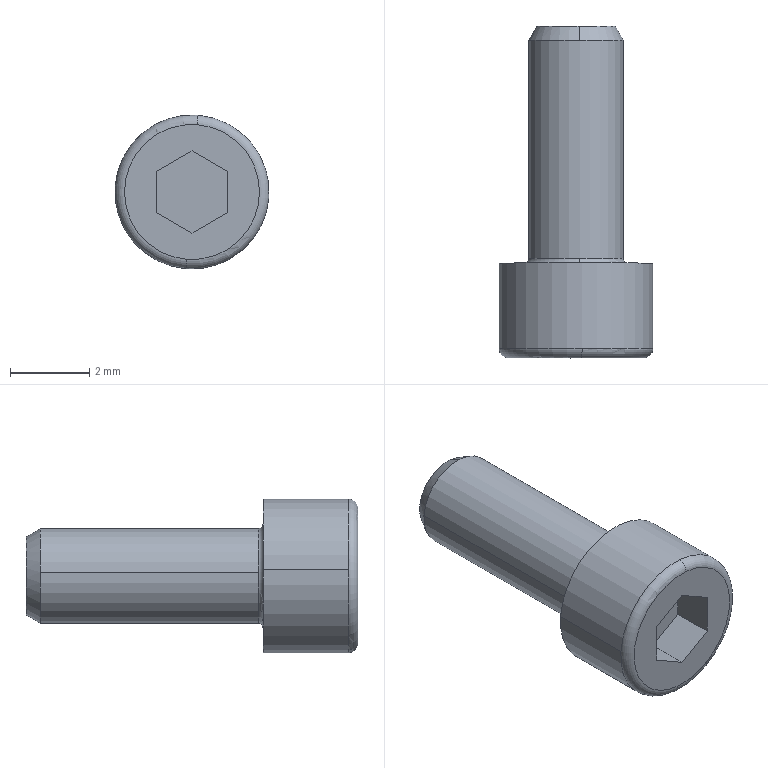Part | STEP file | 2026.6.15-Main Assembly图.sldasm-Part-277 | 1 solid | 20 faces | box 3.9 x 8.4 x 3.9 mm | volume 52.478 mm3 | plane 10 | torus 4 | cylinder 4 | cone 2 | commonest cylinder face diameters 2.4 x2 3.9 x2
STEP:
#1=CARTESIAN_POINT('',(-1526.09,1420.064,3413.556));
#2=VERTEX_POINT('',#1);
#3=CARTESIAN_POINT('',(-1526.09,1420.064,3412.517));
#4=VERTEX_POINT('',#3);
#5=CARTESIAN_POINT('',(-1526.09,1420.064,3413.556));
#6=DIRECTION('',(0.,0.,-1.));
#7=VECTOR('',#6,1000.);
#8=LINE('',#5,#7);
#9=EDGE_CURVE('',#2,#4,#8,.T.);
#10=ORIENTED_EDGE('',*,*,#9,.T.);
#11=CARTESIAN_POINT('',(-1525.19,1420.064,3411.997));
#12=VERTEX_POINT('',#11);
#13=CARTESIAN_POINT('',(-1526.09,1420.064,3412.517));
#14=DIRECTION('',(0.866,0.,-0.5));
#15=VECTOR('',#14,1000.);
#16=LINE('',#13,#15);
#17=EDGE_CURVE('',#4,#12,#16,.T.);
#18=ORIENTED_EDGE('',*,*,#17,.T.);
#19=CARTESIAN_POINT('',(-1524.29,1420.064,3412.517));
#20=VERTEX_POINT('',#19);
#21=CARTESIAN_POINT('',(-1525.19,1420.064,3411.997));
#22=DIRECTION('',(0.866,0.,0.5));
#23=VECTOR('',#22,1000.);
#24=LINE('',#21,#23);
#25=EDGE_CURVE('',#12,#20,#24,.T.);
#26=ORIENTED_EDGE('',*,*,#25,.T.);
#27=CARTESIAN_POINT('',(-1524.29,1420.064,3413.556));
#28=VERTEX_POINT('',#27);
#29=CARTESIAN_POINT('',(-1524.29,1420.064,3412.517));
#30=DIRECTION('',(0.,0.,1.));
#31=VECTOR('',#30,1000.);
#32=LINE('',#29,#31);
#33=EDGE_CURVE('',#20,#28,#32,.T.);
#34=ORIENTED_EDGE('',*,*,#33,.T.);
#35=CARTESIAN_POINT('',(-1525.19,1420.064,3414.076));
#36=VERTEX_POINT('',#35);
#37=CARTESIAN_POINT('',(-1524.29,1420.064,3413.556));
#38=DIRECTION('',(-0.866,0.,0.5));
#39=VECTOR('',#38,1000.);
#40=LINE('',#37,#39);
#41=EDGE_CURVE('',#28,#36,#40,.T.);
#42=ORIENTED_EDGE('',*,*,#41,.T.);
#43=CARTESIAN_POINT('',(-1525.19,1420.064,3414.076));
#44=DIRECTION('',(-0.866,0.,-0.5));
#45=VECTOR('',#44,1000.);
#46=LINE('',#43,#45);
#47=EDGE_CURVE('',#36,#2,#46,.T.);
#48=ORIENTED_EDGE('',*,*,#47,.T.);
#49=EDGE_LOOP('',(#10,#18,#26,#34,#42,#48));
#50=FACE_OUTER_BOUND('',#49,.T.);
#51=CARTESIAN_POINT('',(-1523.39,1420.064,3413.036));
#52=DIRECTION('',(0.,1.,0.));
#53=DIRECTION('',(0.,0.,-1.));
#54=AXIS2_PLACEMENT_3D('',#51,#52,#53);
#55=PLANE('',#54);
#56=ADVANCED_FACE('',(#50),#55,.F.);
#57=ORIENTED_EDGE('',*,*,#9,.F.);
#58=CARTESIAN_POINT('',(-1526.09,1419.014,3413.556));
#59=VERTEX_POINT('',#58);
#60=CARTESIAN_POINT('',(-1526.09,1420.064,3413.556));
#61=DIRECTION('',(0.,-1.,0.));
#62=VECTOR('',#61,1000.);
#63=LINE('',#60,#62);
#64=EDGE_CURVE('',#2,#59,#63,.T.);
#65=ORIENTED_EDGE('',*,*,#64,.T.);
#66=CARTESIAN_POINT('',(-1526.09,1419.014,3412.517));
#67=VERTEX_POINT('',#66);
#68=CARTESIAN_POINT('',(-1526.09,1419.014,3412.517));
#69=DIRECTION('',(0.,0.,1.));
#70=VECTOR('',#69,1000.);
#71=LINE('',#68,#70);
#72=EDGE_CURVE('',#67,#59,#71,.T.);
#73=ORIENTED_EDGE('',*,*,#72,.F.);
#74=CARTESIAN_POINT('',(-1526.09,1420.064,3412.517));
#75=DIRECTION('',(0.,1.,0.));
#76=VECTOR('',#75,1000.);
#77=LINE('',#74,#76);
#78=EDGE_CURVE('',#67,#4,#77,.T.);
#79=ORIENTED_EDGE('',*,*,#78,.T.);
#80=EDGE_LOOP('',(#57,#65,#73,#79));
#81=FACE_OUTER_BOUND('',#80,.T.);
#82=CARTESIAN_POINT('',(-1526.09,1420.064,3413.556));
#83=DIRECTION('',(-1.,0.,0.));
#84=DIRECTION('',(0.,0.,1.));
#85=AXIS2_PLACEMENT_3D('',#82,#83,#84);
#86=PLANE('',#85);
#87=ADVANCED_FACE('',(#81),#86,.F.);
#88=ORIENTED_EDGE('',*,*,#47,.F.);
#89=CARTESIAN_POINT('',(-1525.19,1419.014,3414.076));
#90=VERTEX_POINT('',#89);
#91=CARTESIAN_POINT('',(-1525.19,1420.064,3414.076));
#92=DIRECTION('',(0.,-1.,0.));
#93=VECTOR('',#92,1000.);
#94=LINE('',#91,#93);
#95=EDGE_CURVE('',#36,#90,#94,.T.);
#96=ORIENTED_EDGE('',*,*,#95,.T.);
#97=CARTESIAN_POINT('',(-1526.09,1419.014,3413.556));
#98=DIRECTION('',(0.866,0.,0.5));
#99=VECTOR('',#98,1000.);
#100=LINE('',#97,#99);
#101=EDGE_CURVE('',#59,#90,#100,.T.);
#102=ORIENTED_EDGE('',*,*,#101,.F.);
#103=ORIENTED_EDGE('',*,*,#64,.F.);
#104=EDGE_LOOP('',(#88,#96,#102,#103));
#105=FACE_OUTER_BOUND('',#104,.T.);
#106=CARTESIAN_POINT('',(-1525.19,1420.064,3414.076));
#107=DIRECTION('',(-0.5,0.,0.866));
#108=DIRECTION('',(0.,1.,0.));
#109=AXIS2_PLACEMENT_3D('',#106,#107,#108);
#110=PLANE('',#109);
#111=ADVANCED_FACE('',(#105),#110,.F.);
#112=ORIENTED_EDGE('',*,*,#41,.F.);
#113=CARTESIAN_POINT('',(-1524.29,1419.014,3413.556));
#114=VERTEX_POINT('',#113);
#115=CARTESIAN_POINT('',(-1524.29,1420.064,3413.556));
#116=DIRECTION('',(0.,-1.,0.));
#117=VECTOR('',#116,1000.);
#118=LINE('',#115,#117);
#119=EDGE_CURVE('',#28,#114,#118,.T.);
#120=ORIENTED_EDGE('',*,*,#119,.T.);
#121=CARTESIAN_POINT('',(-1525.19,1419.014,3414.076));
#122=DIRECTION('',(0.866,0.,-0.5));
#123=VECTOR('',#122,1000.);
#124=LINE('',#121,#123);
#125=EDGE_CURVE('',#90,#114,#124,.T.);
#126=ORIENTED_EDGE('',*,*,#125,.F.);
#127=ORIENTED_EDGE('',*,*,#95,.F.);
#128=EDGE_LOOP('',(#112,#120,#126,#127));
#129=FACE_OUTER_BOUND('',#128,.T.);
#130=CARTESIAN_POINT('',(-1524.29,1420.064,3413.556));
#131=DIRECTION('',(0.5,0.,0.866));
#132=DIRECTION('',(-0.866,0.,0.5));
#133=AXIS2_PLACEMENT_3D('',#130,#131,#132);
#134=PLANE('',#133);
#135=ADVANCED_FACE('',(#129),#134,.F.);
#136=ORIENTED_EDGE('',*,*,#33,.F.);
#137=CARTESIAN_POINT('',(-1524.29,1419.014,3412.517));
#138=VERTEX_POINT('',#137);
#139=CARTESIAN_POINT('',(-1524.29,1420.064,3412.517));
#140=DIRECTION('',(0.,-1.,0.));
#141=VECTOR('',#140,1000.);
#142=LINE('',#139,#141);
#143=EDGE_CURVE('',#20,#138,#142,.T.);
#144=ORIENTED_EDGE('',*,*,#143,.T.);
#145=CARTESIAN_POINT('',(-1524.29,1419.014,3413.556));
#146=DIRECTION('',(0.,0.,-1.));
#147=VECTOR('',#146,1000.);
#148=LINE('',#145,#147);
#149=EDGE_CURVE('',#114,#138,#148,.T.);
#150=ORIENTED_EDGE('',*,*,#149,.F.);
#151=ORIENTED_EDGE('',*,*,#119,.F.);
#152=EDGE_LOOP('',(#136,#144,#150,#151));
#153=FACE_OUTER_BOUND('',#152,.T.);
#154=CARTESIAN_POINT('',(-1524.29,1420.064,3412.517));
#155=DIRECTION('',(1.,0.,0.));
#156=DIRECTION('',(0.,0.,1.));
#157=AXIS2_PLACEMENT_3D('',#154,#155,#156);
#158=PLANE('',#157);
#159=ADVANCED_FACE('',(#153),#158,.F.);
#160=ORIENTED_EDGE('',*,*,#25,.F.);
#161=CARTESIAN_POINT('',(-1525.19,1419.014,3411.997));
#162=VERTEX_POINT('',#161);
#163=CARTESIAN_POINT('',(-1525.19,1420.064,3411.997));
#164=DIRECTION('',(0.,-1.,0.));
#165=VECTOR('',#164,1000.);
#166=LINE('',#163,#165);
#167=EDGE_CURVE('',#12,#162,#166,.T.);
#168=ORIENTED_EDGE('',*,*,#167,.T.);
#169=CARTESIAN_POINT('',(-1524.29,1419.014,3412.517));
#170=DIRECTION('',(-0.866,0.,-0.5));
#171=VECTOR('',#170,1000.);
#172=LINE('',#169,#171);
#173=EDGE_CURVE('',#138,#162,#172,.T.);
#174=ORIENTED_EDGE('',*,*,#173,.F.);
#175=ORIENTED_EDGE('',*,*,#143,.F.);
#176=EDGE_LOOP('',(#160,#168,#174,#175));
#177=FACE_OUTER_BOUND('',#176,.T.);
#178=CARTESIAN_POINT('',(-1525.19,1420.064,3411.997));
#179=DIRECTION('',(0.5,0.,-0.866));
#180=DIRECTION('',(0.,-1.,0.));
#181=AXIS2_PLACEMENT_3D('',#178,#179,#180);
#182=PLANE('',#181);
#183=ADVANCED_FACE('',(#177),#182,.F.);
#184=ORIENTED_EDGE('',*,*,#17,.F.);
#185=ORIENTED_EDGE('',*,*,#78,.F.);
#186=CARTESIAN_POINT('',(-1525.19,1419.014,3411.997));
#187=DIRECTION('',(-0.866,0.,0.5));
#188=VECTOR('',#187,1000.);
#189=LINE('',#186,#188);
#190=EDGE_CURVE('',#162,#67,#189,.T.);
#191=ORIENTED_EDGE('',*,*,#190,.F.);
#192=ORIENTED_EDGE('',*,*,#167,.F.);
#193=EDGE_LOOP('',(#184,#185,#191,#192));
#194=FACE_OUTER_BOUND('',#193,.T.);
#195=CARTESIAN_POINT('',(-1526.09,1420.064,3412.517));
#196=DIRECTION('',(-0.5,0.,-0.866));
#197=DIRECTION('',(0.,1.,0.));
#198=AXIS2_PLACEMENT_3D('',#195,#196,#197);
#199=PLANE('',#198);
#200=ADVANCED_FACE('',(#194),#199,.F.);
#201=CARTESIAN_POINT('',(-1525.055,1419.014,3414.741));
#202=VERTEX_POINT('',#201);
#203=CARTESIAN_POINT('',(-1525.324,1419.014,3411.332));
#204=VERTEX_POINT('',#203);
#205=CARTESIAN_POINT('',(-1525.19,1419.014,3413.036));
#206=DIRECTION('',(0.,1.,0.));
#207=DIRECTION('',(0.0785,0.,0.9969));
#208=AXIS2_PLACEMENT_3D('',#205,#206,#207);
#209=CIRCLE('',#208,1.71);
#210=EDGE_CURVE('',#202,#204,#209,.T.);
#211=ORIENTED_EDGE('',*,*,#210,.F.);
#212=CARTESIAN_POINT('',(-1525.19,1419.014,3413.036));
#213=DIRECTION('',(0.,1.,0.));
#214=DIRECTION('',(0.0785,0.,0.9969));
#215=AXIS2_PLACEMENT_3D('',#212,#213,#214);
#216=CIRCLE('',#215,1.71);
#217=EDGE_CURVE('',#204,#202,#216,.T.);
#218=ORIENTED_EDGE('',*,*,#217,.F.);
#219=EDGE_LOOP('',(#211,#218));
#220=FACE_OUTER_BOUND('',#219,.T.);
#221=ORIENTED_EDGE('',*,*,#173,.T.);
#222=ORIENTED_EDGE('',*,*,#190,.T.);
#223=ORIENTED_EDGE('',*,*,#72,.T.);
#224=ORIENTED_EDGE('',*,*,#101,.T.);
#225=ORIENTED_EDGE('',*,*,#125,.T.);
#226=ORIENTED_EDGE('',*,*,#149,.T.);
#227=EDGE_LOOP('',(#221,#222,#223,#224,#225,#226));
#228=FACE_BOUND('',#227,.T.);
#229=CARTESIAN_POINT('',(-1525.19,1419.014,3413.036));
#230=DIRECTION('',(0.,-1.,0.));
#231=DIRECTION('',(-1.,0.,0.));
#232=AXIS2_PLACEMENT_3D('',#229,#230,#231);
#233=PLANE('',#232);
#234=ADVANCED_FACE('',(#220,#228),#233,.T.);
#235=CARTESIAN_POINT('',(-1525.343,1419.254,3411.092));
#236=VERTEX_POINT('',#235);
#237=CARTESIAN_POINT('',(-1525.324,1419.254,3411.332));
#238=DIRECTION('',(0.9969,0.,-0.0785));
#239=DIRECTION('',(0.,1.,0.));
#240=AXIS2_PLACEMENT_3D('',#237,#238,#239);
#241=CIRCLE('',#240,0.24);
#242=EDGE_CURVE('',#204,#236,#241,.T.);
#243=ORIENTED_EDGE('',*,*,#242,.T.);
#244=CARTESIAN_POINT('',(-1523.246,1419.254,3412.883));
#245=VERTEX_POINT('',#244);
#246=CARTESIAN_POINT('',(-1525.19,1419.254,3413.036));
#247=DIRECTION('',(0.,1.,0.));
#248=DIRECTION('',(0.9969,0.,-0.0785));
#249=AXIS2_PLACEMENT_3D('',#246,#247,#248);
#250=CIRCLE('',#249,1.95);
#251=EDGE_CURVE('',#245,#236,#250,.T.);
#252=ORIENTED_EDGE('',*,*,#251,.F.);
#253=CARTESIAN_POINT('',(-1525.036,1419.254,3414.98));
#254=VERTEX_POINT('',#253);
#255=CARTESIAN_POINT('',(-1525.19,1419.254,3413.036));
#256=DIRECTION('',(0.,1.,0.));
#257=DIRECTION('',(0.9969,0.,-0.0785));
#258=AXIS2_PLACEMENT_3D('',#255,#256,#257);
#259=CIRCLE('',#258,1.95);
#260=EDGE_CURVE('',#254,#245,#259,.T.);
#261=ORIENTED_EDGE('',*,*,#260,.F.);
#262=CARTESIAN_POINT('',(-1525.055,1419.254,3414.741));
#263=DIRECTION('',(-0.9969,0.,0.0785));
#264=DIRECTION('',(0.,-1.,0.));
#265=AXIS2_PLACEMENT_3D('',#262,#263,#264);
#266=CIRCLE('',#265,0.24);
#267=EDGE_CURVE('',#202,#254,#266,.T.);
#268=ORIENTED_EDGE('',*,*,#267,.F.);
#269=ORIENTED_EDGE('',*,*,#210,.T.);
#270=EDGE_LOOP('',(#243,#252,#261,#268,#269));
#271=FACE_OUTER_BOUND('',#270,.T.);
#272=CARTESIAN_POINT('',(-1525.19,1419.254,3413.036));
#273=DIRECTION('',(0.,-1.,0.));
#274=DIRECTION('',(-0.0785,0.,-0.9969));
#275=AXIS2_PLACEMENT_3D('',#272,#273,#274);
#276=TOROIDAL_SURFACE('',#275,1.71,0.24);
#277=ADVANCED_FACE('',(#271),#276,.T.);
#278=CARTESIAN_POINT('',(-1527.134,1419.254,3413.189));
#279=VERTEX_POINT('',#278);
#280=CARTESIAN_POINT('',(-1527.134,1421.414,3413.189));
#281=VERTEX_POINT('',#280);
#282=CARTESIAN_POINT('',(-1527.134,1419.014,3413.189));
#283=DIRECTION('',(0.,1.,0.));
#284=VECTOR('',#283,1000.);
#285=LINE('',#282,#284);
#286=EDGE_CURVE('',#279,#281,#285,.T.);
#287=ORIENTED_EDGE('',*,*,#286,.F.);
#288=CARTESIAN_POINT('',(-1525.19,1419.254,3413.036));
#289=DIRECTION('',(0.,1.,0.));
#290=DIRECTION('',(0.9969,0.,-0.0785));
#291=AXIS2_PLACEMENT_3D('',#288,#289,#290);
#292=CIRCLE('',#291,1.95);
#293=EDGE_CURVE('',#279,#254,#292,.T.);
#294=ORIENTED_EDGE('',*,*,#293,.T.);
#295=ORIENTED_EDGE('',*,*,#260,.T.);
#296=CARTESIAN_POINT('',(-1523.246,1421.414,3412.883));
#297=VERTEX_POINT('',#296);
#298=CARTESIAN_POINT('',(-1523.246,1419.014,3412.883));
#299=DIRECTION('',(0.,1.,0.));
#300=VECTOR('',#299,1000.);
#301=LINE('',#298,#300);
#302=EDGE_CURVE('',#245,#297,#301,.T.);
#303=ORIENTED_EDGE('',*,*,#302,.T.);
#304=CARTESIAN_POINT('',(-1525.19,1421.414,3413.036));
#305=DIRECTION('',(0.,1.,0.));
#306=DIRECTION('',(0.9969,0.,-0.0785));
#307=AXIS2_PLACEMENT_3D('',#304,#305,#306);
#308=CIRCLE('',#307,1.95);
#309=EDGE_CURVE('',#281,#297,#308,.T.);
#310=ORIENTED_EDGE('',*,*,#309,.F.);
#311=EDGE_LOOP('',(#287,#294,#295,#303,#310));
#312=FACE_OUTER_BOUND('',#311,.T.);
#313=CARTESIAN_POINT('',(-1525.19,1419.014,3413.036));
#314=DIRECTION('',(0.,1.,0.));
#315=DIRECTION('',(-0.9969,0.,0.0785));
#316=AXIS2_PLACEMENT_3D('',#313,#314,#315);
#317=CYLINDRICAL_SURFACE('',#316,1.95);
#318=ADVANCED_FACE('',(#312),#317,.T.);
#319=CARTESIAN_POINT('',(-1525.19,1421.414,3413.036));
#320=DIRECTION('',(0.,1.,0.));
#321=DIRECTION('',(0.9969,0.,-0.0785));
#322=AXIS2_PLACEMENT_3D('',#319,#320,#321);
#323=CIRCLE('',#322,1.95);
#324=EDGE_CURVE('',#297,#281,#323,.T.);
#325=ORIENTED_EDGE('',*,*,#324,.T.);
#326=ORIENTED_EDGE('',*,*,#309,.T.);
#327=EDGE_LOOP('',(#325,#326));
#328=FACE_OUTER_BOUND('',#327,.T.);
#329=CARTESIAN_POINT('',(-1525.19,1421.414,3414.356));
#330=VERTEX_POINT('',#329);
#331=CARTESIAN_POINT('',(-1525.293,1421.414,3411.72));
#332=VERTEX_POINT('',#331);
#333=CARTESIAN_POINT('',(-1525.19,1421.414,3414.356));
#334=CARTESIAN_POINT('',(-1525.353,1421.414,3414.356));
#335=CARTESIAN_POINT('',(-1525.511,1421.414,3414.327));
#336=CARTESIAN_POINT('',(-1525.682,1421.414,3414.261));
#337=CARTESIAN_POINT('',(-1525.703,1421.414,3414.253));
#338=CARTESIAN_POINT('',(-1525.742,1421.414,3414.235));
#339=CARTESIAN_POINT('',(-1525.801,1421.414,3414.208));
#340=CARTESIAN_POINT('',(-1525.858,1421.414,3414.176));
#341=CARTESIAN_POINT('',(-1525.931,1421.414,3414.129));
#342=CARTESIAN_POINT('',(-1525.968,1421.414,3414.104));
#343=CARTESIAN_POINT('',(-1526.037,1421.414,3414.049));
#344=CARTESIAN_POINT('',(-1526.071,1421.414,3414.02));
#345=CARTESIAN_POINT('',(-1526.167,1421.414,3413.928));
#346=CARTESIAN_POINT('',(-1526.224,1421.414,3413.861));
#347=CARTESIAN_POINT('',(-1526.325,1421.414,3413.715));
#348=CARTESIAN_POINT('',(-1526.366,1421.414,3413.64));
#349=CARTESIAN_POINT('',(-1526.405,1421.414,3413.551));
#350=CARTESIAN_POINT('',(-1526.409,1421.414,3413.541));
#351=CARTESIAN_POINT('',(-1526.418,1421.414,3413.521));
#352=CARTESIAN_POINT('',(-1526.421,1421.414,3413.511));
#353=CARTESIAN_POINT('',(-1526.432,1421.414,3413.483));
#354=CARTESIAN_POINT('',(-1526.452,1421.414,3413.425));
#355=CARTESIAN_POINT('',(-1526.49,1421.414,3413.289));
#356=CARTESIAN_POINT('',(-1526.505,1421.414,3413.17));
#357=CARTESIAN_POINT('',(-1526.512,1421.414,3413.007));
#358=CARTESIAN_POINT('',(-1526.507,1421.414,3412.926));
#359=CARTESIAN_POINT('',(-1526.484,1421.414,3412.766));
#360=CARTESIAN_POINT('',(-1526.461,1421.414,3412.669));
#361=CARTESIAN_POINT('',(-1526.426,1421.414,3412.573));
#362=CARTESIAN_POINT('',(-1526.415,1421.414,3412.545));
#363=CARTESIAN_POINT('',(-1526.41,1421.414,3412.534));
#364=CARTESIAN_POINT('',(-1526.402,1421.414,3412.514));
#365=CARTESIAN_POINT('',(-1526.38,1421.414,3412.465));
#366=CARTESIAN_POINT('',(-1526.356,1421.414,3412.417));
#367=CARTESIAN_POINT('',(-1526.291,1421.414,3412.304));
#368=CARTESIAN_POINT('',(-1526.239,1421.414,3412.231));
#369=CARTESIAN_POINT('',(-1526.123,1421.414,3412.098));
#370=CARTESIAN_POINT('',(-1526.057,1421.414,3412.038));
#371=CARTESIAN_POINT('',(-1525.952,1421.414,3411.958));
#372=CARTESIAN_POINT('',(-1525.915,1421.414,3411.933));
#373=CARTESIAN_POINT('',(-1525.841,1421.414,3411.887));
#374=CARTESIAN_POINT('',(-1525.803,1421.414,3411.867));
#375=CARTESIAN_POINT('',(-1525.725,1421.414,3411.829));
#376=CARTESIAN_POINT('',(-1525.684,1421.414,3411.812));
#377=CARTESIAN_POINT('',(-1525.608,1421.414,3411.784));
#378=CARTESIAN_POINT('',(-1525.493,1421.414,3411.747));
#379=CARTESIAN_POINT('',(-1525.374,1421.414,3411.727));
#380=CARTESIAN_POINT('',(-1525.293,1421.414,3411.72));
#381=B_SPLINE_CURVE_WITH_KNOTS('',3,(#333,#334,#335,#336,#337,#338,#339,#340,#341,#342,#343,#344,#345,#346,#347,#348,#349,#350,#351,#352,#353,#354,#355,#356,#357,#358,#359,#360,#361,#362,#363,#364,#365,#366,#367,#368,#369,#370,#371,#372,#373,#374,#375,#376,#377,#378,#379,#380),.UNSPECIFIED.,.F.,.F.,(4,2,2,1,2,2,2,2,2,2,2,1,1,2,2,1,2,2,1,2,2,2,2,2,2,1,4),(0.,0.125,0.1406,0.1562,0.1875,0.2188,0.25,0.3125,0.375,0.3828,0.3906,0.4063,0.4375,0.5,0.5625,0.625,0.6406,0.6484,0.6563,0.6875,0.75,0.8125,0.8438,0.875,0.9063,0.9375,1.),.UNSPECIFIED.);
#382=EDGE_CURVE('',#330,#332,#381,.T.);
#383=ORIENTED_EDGE('',*,*,#382,.T.);
#384=CARTESIAN_POINT('',(-1525.19,1421.414,3411.716));
#385=VERTEX_POINT('',#384);
#386=CARTESIAN_POINT('',(-1525.293,1421.414,3411.72));
#387=CARTESIAN_POINT('',(-1525.259,1421.414,3411.718));
#388=CARTESIAN_POINT('',(-1525.224,1421.414,3411.716));
#389=CARTESIAN_POINT('',(-1525.19,1421.414,3411.716));
#390=B_SPLINE_CURVE_WITH_KNOTS('',3,(#386,#387,#388,#389),.UNSPECIFIED.,.F.,.F.,(4,4),(0.,1.),.UNSPECIFIED.);
#391=EDGE_CURVE('',#332,#385,#390,.T.);
#392=ORIENTED_EDGE('',*,*,#391,.T.);
#393=CARTESIAN_POINT('',(-1525.086,1421.414,3414.352));
#394=VERTEX_POINT('',#393);
#395=CARTESIAN_POINT('',(-1525.19,1421.414,3411.716));
#396=CARTESIAN_POINT('',(-1525.026,1421.414,3411.716));
#397=CARTESIAN_POINT('',(-1524.868,1421.414,3411.746));
#398=CARTESIAN_POINT('',(-1524.697,1421.414,3411.812));
#399=CARTESIAN_POINT('',(-1524.676,1421.414,3411.82));
#400=CARTESIAN_POINT('',(-1524.637,1421.414,3411.837));
#401=CARTESIAN_POINT('',(-1524.578,1421.414,3411.865));
#402=CARTESIAN_POINT('',(-1524.521,1421.414,3411.897));
#403=CARTESIAN_POINT('',(-1524.448,1421.414,3411.943));
#404=CARTESIAN_POINT('',(-1524.411,1421.414,3411.969));
#405=CARTESIAN_POINT('',(-1524.342,1421.414,3412.024));
#406=CARTESIAN_POINT('',(-1524.308,1421.414,3412.052));
#407=CARTESIAN_POINT('',(-1524.212,1421.414,3412.145));
#408=CARTESIAN_POINT('',(-1524.155,1421.414,3412.212));
#409=CARTESIAN_POINT('',(-1524.054,1421.414,3412.358));
#410=CARTESIAN_POINT('',(-1524.013,1421.414,3412.432));
#411=CARTESIAN_POINT('',(-1523.974,1421.414,3412.522));
#412=CARTESIAN_POINT('',(-1523.97,1421.414,3412.532));
#413=CARTESIAN_POINT('',(-1523.961,1421.414,3412.552));
#414=CARTESIAN_POINT('',(-1523.958,1421.414,3412.562));
#415=CARTESIAN_POINT('',(-1523.947,1421.414,3412.59));
#416=CARTESIAN_POINT('',(-1523.927,1421.414,3412.648));
#417=CARTESIAN_POINT('',(-1523.889,1421.414,3412.783));
#418=CARTESIAN_POINT('',(-1523.874,1421.414,3412.903));
#419=CARTESIAN_POINT('',(-1523.867,1421.414,3413.066));
#420=CARTESIAN_POINT('',(-1523.872,1421.414,3413.147));
#421=CARTESIAN_POINT('',(-1523.895,1421.414,3413.306));
#422=CARTESIAN_POINT('',(-1523.918,1421.414,3413.404));
#423=CARTESIAN_POINT('',(-1523.953,1421.414,3413.5));
#424=CARTESIAN_POINT('',(-1523.965,1421.414,3413.528));
#425=CARTESIAN_POINT('',(-1523.969,1421.414,3413.539));
#426=CARTESIAN_POINT('',(-1523.977,1421.414,3413.558));
#427=CARTESIAN_POINT('',(-1523.999,1421.414,3413.608));
#428=CARTESIAN_POINT('',(-1524.023,1421.414,3413.656));
#429=CARTESIAN_POINT('',(-1524.088,1421.414,3413.769));
#430=CARTESIAN_POINT('',(-1524.14,1421.414,3413.841));
#431=CARTESIAN_POINT('',(-1524.257,1421.414,3413.974));
#432=CARTESIAN_POINT('',(-1524.322,1421.414,3414.035));
#433=CARTESIAN_POINT('',(-1524.427,1421.414,3414.115));
#434=CARTESIAN_POINT('',(-1524.464,1421.414,3414.14));
#435=CARTESIAN_POINT('',(-1524.538,1421.414,3414.185));
#436=CARTESIAN_POINT('',(-1524.576,1421.414,3414.206));
#437=CARTESIAN_POINT('',(-1524.654,1421.414,3414.244));
#438=CARTESIAN_POINT('',(-1524.695,1421.414,3414.261));
#439=CARTESIAN_POINT('',(-1524.771,1421.414,3414.289));
#440=CARTESIAN_POINT('',(-1524.887,1421.414,3414.326));
#441=CARTESIAN_POINT('',(-1525.005,1421.414,3414.346));
#442=CARTESIAN_POINT('',(-1525.086,1421.414,3414.352));
#443=B_SPLINE_CURVE_WITH_KNOTS('',3,(#395,#396,#397,#398,#399,#400,#401,#402,#403,#404,#405,#406,#407,#408,#409,#410,#411,#412,#413,#414,#415,#416,#417,#418,#419,#420,#421,#422,#423,#424,#425,#426,#427,#428,#429,#430,#431,#432,#433,#434,#435,#436,#437,#438,#439,#440,#441,#442),.UNSPECIFIED.,.F.,.F.,(4,2,2,1,2,2,2,2,2,2,2,1,1,2,2,1,2,2,1,2,2,2,2,2,2,1,4),(0.,0.125,0.1406,0.1562,0.1875,0.2187,0.25,0.3125,0.375,0.3828,0.3906,0.4062,0.4375,0.5,0.5625,0.625,0.6406,0.6484,0.6562,0.6875,0.75,0.8125,0.8437,0.875,0.9062,0.9375,1.),.UNSPECIFIED.);
#444=EDGE_CURVE('',#385,#394,#443,.T.);
#445=ORIENTED_EDGE('',*,*,#444,.T.);
#446=CARTESIAN_POINT('',(-1525.086,1421.414,3414.352));
#447=CARTESIAN_POINT('',(-1525.12,1421.414,3414.355));
#448=CARTESIAN_POINT('',(-1525.155,1421.414,3414.356));
#449=CARTESIAN_POINT('',(-1525.19,1421.414,3414.356));
#450=B_SPLINE_CURVE_WITH_KNOTS('',3,(#446,#447,#448,#449),.UNSPECIFIED.,.F.,.F.,(4,4),(0.,1.),.UNSPECIFIED.);
#451=EDGE_CURVE('',#394,#330,#450,.T.);
#452=ORIENTED_EDGE('',*,*,#451,.T.);
#453=EDGE_LOOP('',(#383,#392,#445,#452));
#454=FACE_BOUND('',#453,.T.);
#455=CARTESIAN_POINT('',(-1527.14,1421.414,3413.036));
#456=DIRECTION('',(0.,1.,0.));
#457=DIRECTION('',(0.,0.,-1.));
#458=AXIS2_PLACEMENT_3D('',#455,#456,#457);
#459=PLANE('',#458);
#460=ADVANCED_FACE('',(#328,#454),#459,.T.);
#461=CARTESIAN_POINT('',(-1525.112,1427.414,3414.025));
#462=VERTEX_POINT('',#461);
#463=CARTESIAN_POINT('',(-1525.267,1427.414,3412.047));
#464=VERTEX_POINT('',#463);
#465=CARTESIAN_POINT('',(-1525.19,1427.414,3413.036));
#466=DIRECTION('',(0.,-1.,0.));
#467=DIRECTION('',(0.0785,0.,0.9969));
#468=AXIS2_PLACEMENT_3D('',#465,#466,#467);
#469=CIRCLE('',#468,0.9922);
#470=EDGE_CURVE('',#462,#464,#469,.T.);
#471=ORIENTED_EDGE('',*,*,#470,.F.);
#472=CARTESIAN_POINT('',(-1525.19,1427.414,3413.036));
#473=DIRECTION('',(0.,-1.,0.));
#474=DIRECTION('',(0.0785,0.,0.9969));
#475=AXIS2_PLACEMENT_3D('',#472,#473,#474);
#476=CIRCLE('',#475,0.9922);
#477=EDGE_CURVE('',#464,#462,#476,.T.);
#478=ORIENTED_EDGE('',*,*,#477,.F.);
#479=EDGE_LOOP('',(#471,#478));
#480=FACE_OUTER_BOUND('',#479,.T.);
#481=CARTESIAN_POINT('',(-1526.39,1427.414,3413.036));
#482=DIRECTION('',(0.,1.,0.));
#483=DIRECTION('',(0.,0.,-1.));
#484=AXIS2_PLACEMENT_3D('',#481,#482,#483);
#485=PLANE('',#484);
#486=ADVANCED_FACE('',(#480),#485,.T.);
#487=CARTESIAN_POINT('',(-1525.095,1421.534,3414.233));
#488=VERTEX_POINT('',#487);
#489=CARTESIAN_POINT('',(-1525.086,1421.534,3414.352));
#490=DIRECTION('',(-0.9969,0.,0.0785));
#491=DIRECTION('',(0.,1.,0.));
#492=AXIS2_PLACEMENT_3D('',#489,#490,#491);
#493=CIRCLE('',#492,0.12);
#494=EDGE_CURVE('',#488,#394,#493,.T.);
#495=ORIENTED_EDGE('',*,*,#494,.F.);
#496=CARTESIAN_POINT('',(-1526.386,1421.534,3413.131));
#497=VERTEX_POINT('',#496);
#498=CARTESIAN_POINT('',(-1525.19,1421.534,3413.036));
#499=DIRECTION('',(0.,1.,0.));
#500=DIRECTION('',(0.9969,0.,-0.0785));
#501=AXIS2_PLACEMENT_3D('',#498,#499,#500);
#502=CIRCLE('',#501,1.2);
#503=EDGE_CURVE('',#497,#488,#502,.T.);
#504=ORIENTED_EDGE('',*,*,#503,.F.);
#505=CARTESIAN_POINT('',(-1525.284,1421.534,3411.84));
#506=VERTEX_POINT('',#505);
#507=CARTESIAN_POINT('',(-1525.19,1421.534,3413.036));
#508=DIRECTION('',(0.,1.,0.));
#509=DIRECTION('',(0.9969,0.,-0.0785));
#510=AXIS2_PLACEMENT_3D('',#507,#508,#509);
#511=CIRCLE('',#510,1.2);
#512=EDGE_CURVE('',#506,#497,#511,.T.);
#513=ORIENTED_EDGE('',*,*,#512,.F.);
#514=CARTESIAN_POINT('',(-1525.293,1421.534,3411.72));
#515=DIRECTION('',(0.9969,0.,-0.0785));
#516=DIRECTION('',(0.,-1.,0.));
#517=AXIS2_PLACEMENT_3D('',#514,#515,#516);
#518=CIRCLE('',#517,0.12);
#519=EDGE_CURVE('',#506,#332,#518,.T.);
#520=ORIENTED_EDGE('',*,*,#519,.T.);
#521=ORIENTED_EDGE('',*,*,#382,.F.);
#522=ORIENTED_EDGE('',*,*,#451,.F.);
#523=EDGE_LOOP('',(#495,#504,#513,#520,#521,#522));
#524=FACE_OUTER_BOUND('',#523,.T.);
#525=CARTESIAN_POINT('',(-1525.19,1421.534,3413.036));
#526=DIRECTION('',(0.,1.,0.));
#527=DIRECTION('',(0.0785,0.,0.9969));
#528=AXIS2_PLACEMENT_3D('',#525,#526,#527);
#529=TOROIDAL_SURFACE('',#528,1.32,0.12);
#530=ADVANCED_FACE('',(#524),#529,.F.);
#531=CARTESIAN_POINT('',(-1525.284,1427.054,3411.84));
#532=VERTEX_POINT('',#531);
#533=CARTESIAN_POINT('',(-1525.284,1427.054,3411.84));
#534=DIRECTION('',(0.03925,0.866,0.4985));
#535=VECTOR('',#534,1000.);
#536=LINE('',#533,#535);
#537=EDGE_CURVE('',#532,#464,#536,.T.);
#538=ORIENTED_EDGE('',*,*,#537,.T.);
#539=ORIENTED_EDGE('',*,*,#477,.T.);
#540=CARTESIAN_POINT('',(-1525.095,1427.054,3414.233));
#541=VERTEX_POINT('',#540);
#542=CARTESIAN_POINT('',(-1525.095,1427.054,3414.233));
#543=DIRECTION('',(-0.03925,0.866,-0.4985));
#544=VECTOR('',#543,1000.);
#545=LINE('',#542,#544);
#546=EDGE_CURVE('',#541,#462,#545,.T.);
#547=ORIENTED_EDGE('',*,*,#546,.F.);
#548=CARTESIAN_POINT('',(-1523.993,1427.054,3412.942));
#549=VERTEX_POINT('',#548);
#550=CARTESIAN_POINT('',(-1525.19,1427.054,3413.036));
#551=DIRECTION('',(0.,-1.,0.));
#552=DIRECTION('',(0.9969,0.,-0.0785));
#553=AXIS2_PLACEMENT_3D('',#550,#551,#552);
#554=CIRCLE('',#553,1.2);
#555=EDGE_CURVE('',#549,#541,#554,.T.);
#556=ORIENTED_EDGE('',*,*,#555,.F.);
#557=CARTESIAN_POINT('',(-1525.19,1427.054,3413.036));
#558=DIRECTION('',(0.,-1.,0.));
#559=DIRECTION('',(0.9969,0.,-0.0785));
#560=AXIS2_PLACEMENT_3D('',#557,#558,#559);
#561=CIRCLE('',#560,1.2);
#562=EDGE_CURVE('',#532,#549,#561,.T.);
#563=ORIENTED_EDGE('',*,*,#562,.F.);
#564=EDGE_LOOP('',(#538,#539,#547,#556,#563));
#565=FACE_OUTER_BOUND('',#564,.T.);
#566=CARTESIAN_POINT('',(-1525.19,1427.054,3413.036));
#567=DIRECTION('',(0.,-1.,0.));
#568=DIRECTION('',(-0.0785,0.,-0.9969));
#569=AXIS2_PLACEMENT_3D('',#566,#567,#568);
#570=CONICAL_SURFACE('',#569,1.2,0.5236);
#571=ADVANCED_FACE('',(#565),#570,.T.);
#572=CARTESIAN_POINT('',(-1526.386,1427.054,3413.131));
#573=VERTEX_POINT('',#572);
#574=CARTESIAN_POINT('',(-1526.386,1419.014,3413.131));
#575=DIRECTION('',(0.,1.,0.));
#576=VECTOR('',#575,1000.);
#577=LINE('',#574,#576);
#578=EDGE_CURVE('',#497,#573,#577,.T.);
#579=ORIENTED_EDGE('',*,*,#578,.F.);
#580=ORIENTED_EDGE('',*,*,#503,.T.);
#581=CARTESIAN_POINT('',(-1523.993,1421.534,3412.942));
#582=VERTEX_POINT('',#581);
#583=CARTESIAN_POINT('',(-1525.19,1421.534,3413.036));
#584=DIRECTION('',(0.,1.,0.));
#585=DIRECTION('',(0.9969,0.,-0.0785));
#586=AXIS2_PLACEMENT_3D('',#583,#584,#585);
#587=CIRCLE('',#586,1.2);
#588=EDGE_CURVE('',#488,#582,#587,.T.);
#589=ORIENTED_EDGE('',*,*,#588,.T.);
#590=CARTESIAN_POINT('',(-1523.993,1419.014,3412.942));
#591=DIRECTION('',(0.,1.,0.));
#592=VECTOR('',#591,1000.);
#593=LINE('',#590,#592);
#594=EDGE_CURVE('',#582,#549,#593,.T.);
#595=ORIENTED_EDGE('',*,*,#594,.T.);
#596=ORIENTED_EDGE('',*,*,#555,.T.);
#597=CARTESIAN_POINT('',(-1525.19,1427.054,3413.036));
#598=DIRECTION('',(0.,-1.,0.));
#599=DIRECTION('',(0.9969,0.,-0.0785));
#600=AXIS2_PLACEMENT_3D('',#597,#598,#599);
#601=CIRCLE('',#600,1.2);
#602=EDGE_CURVE('',#541,#573,#601,.T.);
#603=ORIENTED_EDGE('',*,*,#602,.T.);
#604=EDGE_LOOP('',(#579,#580,#589,#595,#596,#603));
#605=FACE_OUTER_BOUND('',#604,.T.);
#606=CARTESIAN_POINT('',(-1525.19,1419.014,3413.036));
#607=DIRECTION('',(0.,1.,0.));
#608=DIRECTION('',(-0.9969,0.,0.0785));
#609=AXIS2_PLACEMENT_3D('',#606,#607,#608);
#610=CYLINDRICAL_SURFACE('',#609,1.2);
#611=ADVANCED_FACE('',(#605),#610,.T.);
#612=CARTESIAN_POINT('',(-1525.19,1419.254,3413.036));
#613=DIRECTION('',(0.,1.,0.));
#614=DIRECTION('',(0.9969,0.,-0.0785));
#615=AXIS2_PLACEMENT_3D('',#612,#613,#614);
#616=CIRCLE('',#615,1.95);
#617=EDGE_CURVE('',#236,#279,#616,.T.);
#618=ORIENTED_EDGE('',*,*,#617,.F.);
#619=ORIENTED_EDGE('',*,*,#242,.F.);
#620=ORIENTED_EDGE('',*,*,#217,.T.);
#621=ORIENTED_EDGE('',*,*,#267,.T.);
#622=ORIENTED_EDGE('',*,*,#293,.F.);
#623=EDGE_LOOP('',(#618,#619,#620,#621,#622));
#624=FACE_OUTER_BOUND('',#623,.T.);
#625=CARTESIAN_POINT('',(-1525.19,1419.254,3413.036));
#626=DIRECTION('',(0.,-1.,0.));
#627=DIRECTION('',(-0.0785,0.,-0.9969));
#628=AXIS2_PLACEMENT_3D('',#625,#626,#627);
#629=TOROIDAL_SURFACE('',#628,1.71,0.24);
#630=ADVANCED_FACE('',(#624),#629,.T.);
#631=ORIENTED_EDGE('',*,*,#617,.T.);
#632=ORIENTED_EDGE('',*,*,#286,.T.);
#633=ORIENTED_EDGE('',*,*,#324,.F.);
#634=ORIENTED_EDGE('',*,*,#302,.F.);
#635=ORIENTED_EDGE('',*,*,#251,.T.);
#636=EDGE_LOOP('',(#631,#632,#633,#634,#635));
#637=FACE_OUTER_BOUND('',#636,.T.);
#638=CARTESIAN_POINT('',(-1525.19,1419.014,3413.036));
#639=DIRECTION('',(0.,1.,0.));
#640=DIRECTION('',(-0.9969,0.,0.0785));
#641=AXIS2_PLACEMENT_3D('',#638,#639,#640);
#642=CYLINDRICAL_SURFACE('',#641,1.95);
#643=ADVANCED_FACE('',(#637),#642,.T.);
#644=ORIENTED_EDGE('',*,*,#588,.F.);
#645=ORIENTED_EDGE('',*,*,#494,.T.);
#646=ORIENTED_EDGE('',*,*,#444,.F.);
#647=ORIENTED_EDGE('',*,*,#391,.F.);
#648=ORIENTED_EDGE('',*,*,#519,.F.);
#649=CARTESIAN_POINT('',(-1525.19,1421.534,3413.036));
#650=DIRECTION('',(0.,1.,0.));
#651=DIRECTION('',(0.9969,0.,-0.0785));
#652=AXIS2_PLACEMENT_3D('',#649,#650,#651);
#653=CIRCLE('',#652,1.2);
#654=EDGE_CURVE('',#582,#506,#653,.T.);
#655=ORIENTED_EDGE('',*,*,#654,.F.);
#656=EDGE_LOOP('',(#644,#645,#646,#647,#648,#655));
#657=FACE_OUTER_BOUND('',#656,.T.);
#658=CARTESIAN_POINT('',(-1525.19,1421.534,3413.036));
#659=DIRECTION('',(0.,1.,0.));
#660=DIRECTION('',(0.0785,0.,0.9969));
#661=AXIS2_PLACEMENT_3D('',#658,#659,#660);
#662=TOROIDAL_SURFACE('',#661,1.32,0.12);
#663=ADVANCED_FACE('',(#657),#662,.F.);
#664=ORIENTED_EDGE('',*,*,#470,.T.);
#665=ORIENTED_EDGE('',*,*,#537,.F.);
#666=CARTESIAN_POINT('',(-1525.19,1427.054,3413.036));
#667=DIRECTION('',(0.,-1.,0.));
#668=DIRECTION('',(0.9969,0.,-0.0785));
#669=AXIS2_PLACEMENT_3D('',#666,#667,#668);
#670=CIRCLE('',#669,1.2);
#671=EDGE_CURVE('',#573,#532,#670,.T.);
#672=ORIENTED_EDGE('',*,*,#671,.F.);
#673=ORIENTED_EDGE('',*,*,#602,.F.);
#674=ORIENTED_EDGE('',*,*,#546,.T.);
#675=EDGE_LOOP('',(#664,#665,#672,#673,#674));
#676=FACE_OUTER_BOUND('',#675,.T.);
#677=CARTESIAN_POINT('',(-1525.19,1427.054,3413.036));
#678=DIRECTION('',(0.,-1.,0.));
#679=DIRECTION('',(-0.0785,0.,-0.9969));
#680=AXIS2_PLACEMENT_3D('',#677,#678,#679);
#681=CONICAL_SURFACE('',#680,1.2,0.5236);
#682=ADVANCED_FACE('',(#676),#681,.T.);
#683=ORIENTED_EDGE('',*,*,#512,.T.);
#684=ORIENTED_EDGE('',*,*,#578,.T.);
#685=ORIENTED_EDGE('',*,*,#671,.T.);
#686=ORIENTED_EDGE('',*,*,#562,.T.);
#687=ORIENTED_EDGE('',*,*,#594,.F.);
#688=ORIENTED_EDGE('',*,*,#654,.T.);
#689=EDGE_LOOP('',(#683,#684,#685,#686,#687,#688));
#690=FACE_OUTER_BOUND('',#689,.T.);
#691=CARTESIAN_POINT('',(-1525.19,1419.014,3413.036));
#692=DIRECTION('',(0.,1.,0.));
#693=DIRECTION('',(-0.9969,0.,0.0785));
#694=AXIS2_PLACEMENT_3D('',#691,#692,#693);
#695=CYLINDRICAL_SURFACE('',#694,1.2);
#696=ADVANCED_FACE('',(#690),#695,.T.);
#697=CLOSED_SHELL('',(#56,#87,#111,#135,#159,#183,#200,#234,#277,#318,#460,#486,#530,#571,#611,#630,#643,#663,#682,#696));
#698=MANIFOLD_SOLID_BREP('',#697);
#699=CARTESIAN_POINT('',(0.,0.,0.));
#700=DIRECTION('',(0.,0.,1.));
#701=DIRECTION('',(1.,0.,0.));
#702=AXIS2_PLACEMENT_3D('',#699,#700,#701);
#703=(LENGTH_UNIT()NAMED_UNIT(*)SI_UNIT(.MILLI.,.METRE.));
#704=UNCERTAINTY_MEASURE_WITH_UNIT(LENGTH_MEASURE(0.00001),#703,'','');
#705=(NAMED_UNIT(*)PLANE_ANGLE_UNIT()SI_UNIT($,.RADIAN.));
#706=(NAMED_UNIT(*)SI_UNIT($,.STERADIAN.)SOLID_ANGLE_UNIT());
#707=(GEOMETRIC_REPRESENTATION_CONTEXT(3)GLOBAL_UNCERTAINTY_ASSIGNED_CONTEXT((#704))GLOBAL_UNIT_ASSIGNED_CONTEXT((#703,#705,#706))REPRESENTATION_CONTEXT('',''));
#708=ADVANCED_BREP_SHAPE_REPRESENTATION('',(#698,#702),#707);